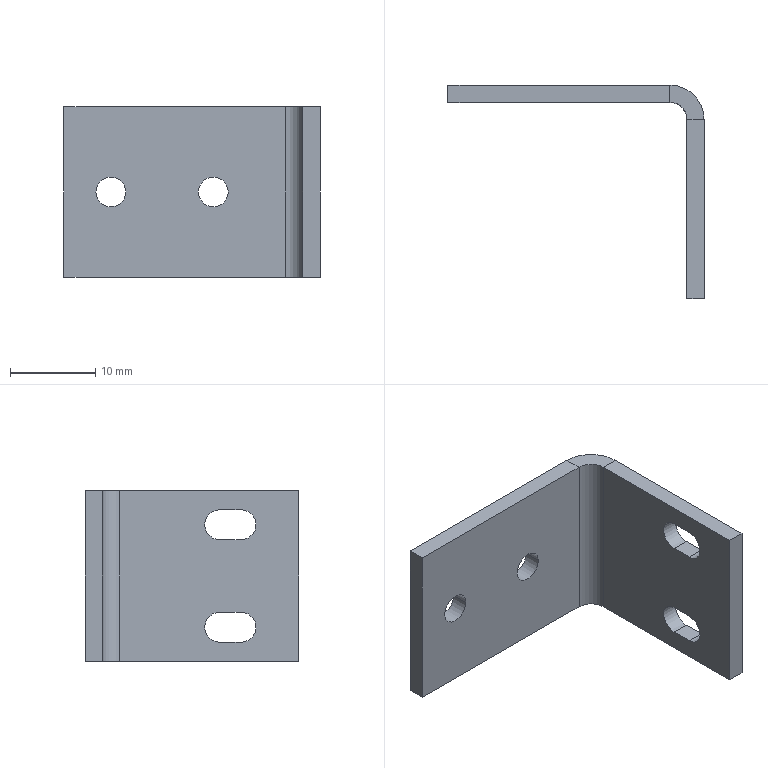Part | STEP file | Cup gripper lift proximity switch bracket 01V1.201001 | 1 solid | 26 faces | box 30 x 25 x 20 mm | volume 1957 mm3 | plane 16 | cylinder 10 | commonest cylinder face diameters 3.5 x8 4 x1 8 x1